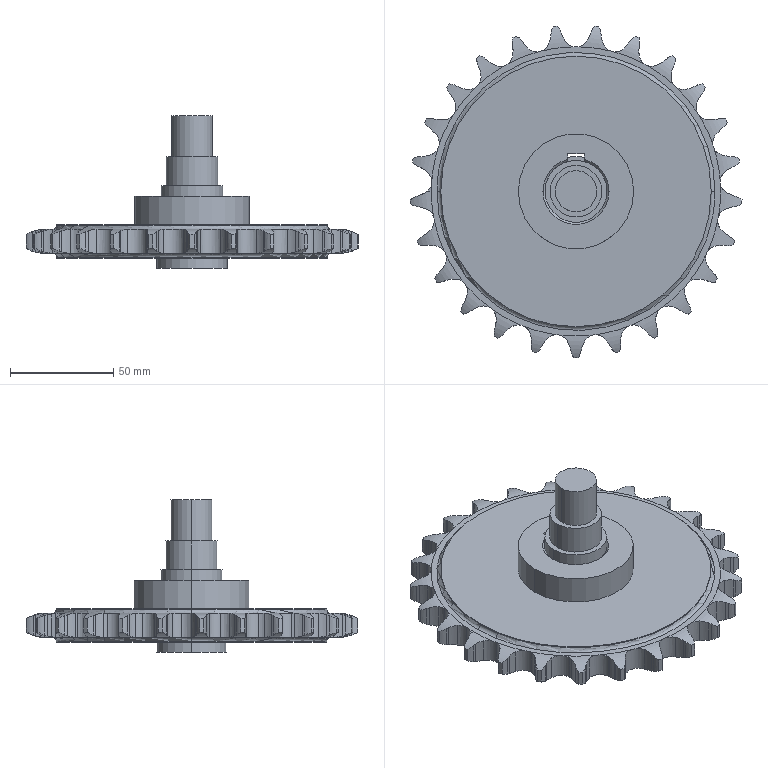Part | NX | features BREP 2 | 2 solids | 303 faces | box 160.793 x 160.481 x 74 mm | volume 314887 mm3 | cylinder 179 | plane 63 | torus 56 | cone 5 | commonest cylinder face diameters 17.202 x53 31.126 x52 12.07 x32 161 x25 30 x5 131 x4